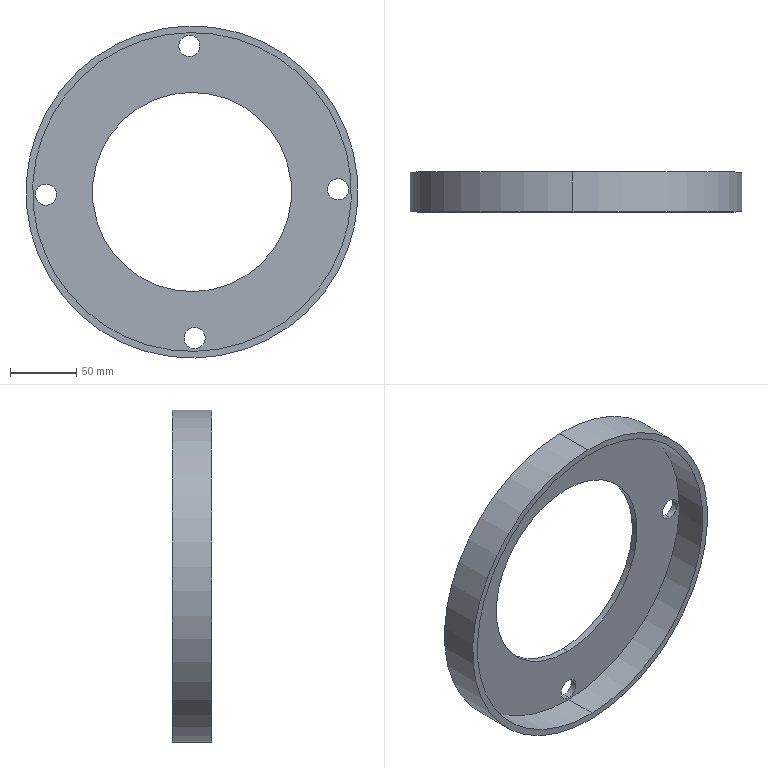Part | STEP file | 2026.6.15-Main Assembly图.sldasm-Part-1 | 1 solid | 17 faces | box 250 x 30 x 250 mm | volume 249270 mm3 | cylinder 14 | plane 3 | commonest cylinder face diameters 16 x8 150 x2 240 x2 250 x2
STEP:
#1=CARTESIAN_POINT('',(-752.482,776.976,3092.657));
#2=VERTEX_POINT('',#1);
#3=CARTESIAN_POINT('',(-752.191,776.976,3076.66));
#4=VERTEX_POINT('',#3);
#5=CARTESIAN_POINT('',(-752.337,776.976,3084.658));
#6=DIRECTION('',(0.,-1.,0.));
#7=DIRECTION('',(0.01819,0.,-0.9998));
#8=AXIS2_PLACEMENT_3D('',#5,#6,#7);
#9=CIRCLE('',#8,8.);
#10=EDGE_CURVE('',#2,#4,#9,.T.);
#11=ORIENTED_EDGE('',*,*,#10,.T.);
#12=CARTESIAN_POINT('',(-752.191,781.976,3076.66));
#13=VERTEX_POINT('',#12);
#14=CARTESIAN_POINT('',(-752.191,756.976,3076.66));
#15=DIRECTION('',(0.,-1.,0.));
#16=VECTOR('',#15,1000.);
#17=LINE('',#14,#16);
#18=EDGE_CURVE('',#13,#4,#17,.T.);
#19=ORIENTED_EDGE('',*,*,#18,.F.);
#20=CARTESIAN_POINT('',(-752.482,781.976,3092.657));
#21=VERTEX_POINT('',#20);
#22=CARTESIAN_POINT('',(-752.337,781.976,3084.658));
#23=DIRECTION('',(0.,1.,0.));
#24=DIRECTION('',(-0.01819,0.,0.9998));
#25=AXIS2_PLACEMENT_3D('',#22,#23,#24);
#26=CIRCLE('',#25,8.);
#27=EDGE_CURVE('',#13,#21,#26,.T.);
#28=ORIENTED_EDGE('',*,*,#27,.T.);
#29=CARTESIAN_POINT('',(-752.482,756.976,3092.657));
#30=DIRECTION('',(0.,-1.,0.));
#31=VECTOR('',#30,1000.);
#32=LINE('',#29,#31);
#33=EDGE_CURVE('',#21,#2,#32,.T.);
#34=ORIENTED_EDGE('',*,*,#33,.T.);
#35=EDGE_LOOP('',(#11,#19,#28,#34));
#36=FACE_OUTER_BOUND('',#35,.T.);
#37=CARTESIAN_POINT('',(-752.337,756.976,3084.658));
#38=DIRECTION('',(0.,1.,0.));
#39=DIRECTION('',(0.01819,0.,-0.9998));
#40=AXIS2_PLACEMENT_3D('',#37,#38,#39);
#41=CYLINDRICAL_SURFACE('',#40,8.);
#42=ADVANCED_FACE('',(#36),#41,.F.);
#43=CARTESIAN_POINT('',(-644.501,776.976,3204.639));
#44=VERTEX_POINT('',#43);
#45=CARTESIAN_POINT('',(-644.21,776.976,3188.642));
#46=VERTEX_POINT('',#45);
#47=CARTESIAN_POINT('',(-644.356,776.976,3196.641));
#48=DIRECTION('',(0.,-1.,0.));
#49=DIRECTION('',(0.01819,0.,-0.9998));
#50=AXIS2_PLACEMENT_3D('',#47,#48,#49);
#51=CIRCLE('',#50,8.);
#52=EDGE_CURVE('',#44,#46,#51,.T.);
#53=ORIENTED_EDGE('',*,*,#52,.T.);
#54=CARTESIAN_POINT('',(-644.21,781.976,3188.642));
#55=VERTEX_POINT('',#54);
#56=CARTESIAN_POINT('',(-644.21,756.976,3188.642));
#57=DIRECTION('',(0.,-1.,0.));
#58=VECTOR('',#57,1000.);
#59=LINE('',#56,#58);
#60=EDGE_CURVE('',#55,#46,#59,.T.);
#61=ORIENTED_EDGE('',*,*,#60,.F.);
#62=CARTESIAN_POINT('',(-644.501,781.976,3204.639));
#63=VERTEX_POINT('',#62);
#64=CARTESIAN_POINT('',(-644.356,781.976,3196.641));
#65=DIRECTION('',(0.,1.,0.));
#66=DIRECTION('',(-0.01819,0.,0.9998));
#67=AXIS2_PLACEMENT_3D('',#64,#65,#66);
#68=CIRCLE('',#67,8.);
#69=EDGE_CURVE('',#55,#63,#68,.T.);
#70=ORIENTED_EDGE('',*,*,#69,.T.);
#71=CARTESIAN_POINT('',(-644.501,756.976,3204.639));
#72=DIRECTION('',(0.,-1.,0.));
#73=VECTOR('',#72,1000.);
#74=LINE('',#71,#73);
#75=EDGE_CURVE('',#63,#44,#74,.T.);
#76=ORIENTED_EDGE('',*,*,#75,.T.);
#77=EDGE_LOOP('',(#53,#61,#70,#76));
#78=FACE_OUTER_BOUND('',#77,.T.);
#79=CARTESIAN_POINT('',(-644.356,756.976,3196.641));
#80=DIRECTION('',(0.,1.,0.));
#81=DIRECTION('',(0.01819,0.,-0.9998));
#82=AXIS2_PLACEMENT_3D('',#79,#80,#81);
#83=CYLINDRICAL_SURFACE('',#82,8.);
#84=ADVANCED_FACE('',(#78),#83,.F.);
#85=CARTESIAN_POINT('',(-864.465,776.976,3200.638));
#86=VERTEX_POINT('',#85);
#87=CARTESIAN_POINT('',(-864.174,776.976,3184.641));
#88=VERTEX_POINT('',#87);
#89=CARTESIAN_POINT('',(-864.319,776.976,3192.639));
#90=DIRECTION('',(0.,-1.,0.));
#91=DIRECTION('',(0.01819,0.,-0.9998));
#92=AXIS2_PLACEMENT_3D('',#89,#90,#91);
#93=CIRCLE('',#92,8.);
#94=EDGE_CURVE('',#86,#88,#93,.T.);
#95=ORIENTED_EDGE('',*,*,#94,.T.);
#96=CARTESIAN_POINT('',(-864.174,781.976,3184.641));
#97=VERTEX_POINT('',#96);
#98=CARTESIAN_POINT('',(-864.174,756.976,3184.641));
#99=DIRECTION('',(0.,-1.,0.));
#100=VECTOR('',#99,1000.);
#101=LINE('',#98,#100);
#102=EDGE_CURVE('',#97,#88,#101,.T.);
#103=ORIENTED_EDGE('',*,*,#102,.F.);
#104=CARTESIAN_POINT('',(-864.465,781.976,3200.638));
#105=VERTEX_POINT('',#104);
#106=CARTESIAN_POINT('',(-864.319,781.976,3192.639));
#107=DIRECTION('',(0.,1.,0.));
#108=DIRECTION('',(0.01819,0.,-0.9998));
#109=AXIS2_PLACEMENT_3D('',#106,#107,#108);
#110=CIRCLE('',#109,8.);
#111=EDGE_CURVE('',#97,#105,#110,.T.);
#112=ORIENTED_EDGE('',*,*,#111,.T.);
#113=CARTESIAN_POINT('',(-864.465,756.976,3200.638));
#114=DIRECTION('',(0.,-1.,0.));
#115=VECTOR('',#114,1000.);
#116=LINE('',#113,#115);
#117=EDGE_CURVE('',#105,#86,#116,.T.);
#118=ORIENTED_EDGE('',*,*,#117,.T.);
#119=EDGE_LOOP('',(#95,#103,#112,#118));
#120=FACE_OUTER_BOUND('',#119,.T.);
#121=CARTESIAN_POINT('',(-864.319,756.976,3192.639));
#122=DIRECTION('',(0.,1.,0.));
#123=DIRECTION('',(0.01819,0.,-0.9998));
#124=AXIS2_PLACEMENT_3D('',#121,#122,#123);
#125=CYLINDRICAL_SURFACE('',#124,8.);
#126=ADVANCED_FACE('',(#120),#125,.F.);
#127=CARTESIAN_POINT('',(-756.484,776.976,3312.621));
#128=VERTEX_POINT('',#127);
#129=CARTESIAN_POINT('',(-756.193,776.976,3296.623));
#130=VERTEX_POINT('',#129);
#131=CARTESIAN_POINT('',(-756.338,776.976,3304.622));
#132=DIRECTION('',(0.,-1.,0.));
#133=DIRECTION('',(0.01819,0.,-0.9998));
#134=AXIS2_PLACEMENT_3D('',#131,#132,#133);
#135=CIRCLE('',#134,8.);
#136=EDGE_CURVE('',#128,#130,#135,.T.);
#137=ORIENTED_EDGE('',*,*,#136,.T.);
#138=CARTESIAN_POINT('',(-756.193,781.976,3296.623));
#139=VERTEX_POINT('',#138);
#140=CARTESIAN_POINT('',(-756.193,756.976,3296.623));
#141=DIRECTION('',(0.,-1.,0.));
#142=VECTOR('',#141,1000.);
#143=LINE('',#140,#142);
#144=EDGE_CURVE('',#139,#130,#143,.T.);
#145=ORIENTED_EDGE('',*,*,#144,.F.);
#146=CARTESIAN_POINT('',(-756.484,781.976,3312.621));
#147=VERTEX_POINT('',#146);
#148=CARTESIAN_POINT('',(-756.338,781.976,3304.622));
#149=DIRECTION('',(0.,1.,0.));
#150=DIRECTION('',(0.01819,0.,-0.9998));
#151=AXIS2_PLACEMENT_3D('',#148,#149,#150);
#152=CIRCLE('',#151,8.);
#153=EDGE_CURVE('',#139,#147,#152,.T.);
#154=ORIENTED_EDGE('',*,*,#153,.T.);
#155=CARTESIAN_POINT('',(-756.484,756.976,3312.621));
#156=DIRECTION('',(0.,-1.,0.));
#157=VECTOR('',#156,1000.);
#158=LINE('',#155,#157);
#159=EDGE_CURVE('',#147,#128,#158,.T.);
#160=ORIENTED_EDGE('',*,*,#159,.T.);
#161=EDGE_LOOP('',(#137,#145,#154,#160));
#162=FACE_OUTER_BOUND('',#161,.T.);
#163=CARTESIAN_POINT('',(-756.338,756.976,3304.622));
#164=DIRECTION('',(0.,1.,0.));
#165=DIRECTION('',(0.01819,0.,-0.9998));
#166=AXIS2_PLACEMENT_3D('',#163,#164,#165);
#167=CYLINDRICAL_SURFACE('',#166,8.);
#168=ADVANCED_FACE('',(#162),#167,.F.);
#169=CARTESIAN_POINT('',(-756.52,776.976,3314.62));
#170=VERTEX_POINT('',#169);
#171=CARTESIAN_POINT('',(-752.155,776.976,3074.66));
#172=VERTEX_POINT('',#171);
#173=CARTESIAN_POINT('',(-754.337,776.976,3194.64));
#174=DIRECTION('',(0.,-1.,0.));
#175=DIRECTION('',(0.01819,0.,-0.9998));
#176=AXIS2_PLACEMENT_3D('',#173,#174,#175);
#177=CIRCLE('',#176,120.);
#178=EDGE_CURVE('',#170,#172,#177,.T.);
#179=ORIENTED_EDGE('',*,*,#178,.F.);
#180=CARTESIAN_POINT('',(-756.52,751.976,3314.62));
#181=VERTEX_POINT('',#180);
#182=CARTESIAN_POINT('',(-756.52,776.976,3314.62));
#183=DIRECTION('',(0.,-1.,0.));
#184=VECTOR('',#183,1000.);
#185=LINE('',#182,#184);
#186=EDGE_CURVE('',#170,#181,#185,.T.);
#187=ORIENTED_EDGE('',*,*,#186,.T.);
#188=CARTESIAN_POINT('',(-752.155,751.976,3074.66));
#189=VERTEX_POINT('',#188);
#190=CARTESIAN_POINT('',(-754.337,751.976,3194.64));
#191=DIRECTION('',(0.,-1.,0.));
#192=DIRECTION('',(0.01819,0.,-0.9998));
#193=AXIS2_PLACEMENT_3D('',#190,#191,#192);
#194=CIRCLE('',#193,120.);
#195=EDGE_CURVE('',#181,#189,#194,.T.);
#196=ORIENTED_EDGE('',*,*,#195,.T.);
#197=CARTESIAN_POINT('',(-752.155,776.976,3074.66));
#198=DIRECTION('',(0.,-1.,0.));
#199=VECTOR('',#198,1000.);
#200=LINE('',#197,#199);
#201=EDGE_CURVE('',#172,#189,#200,.T.);
#202=ORIENTED_EDGE('',*,*,#201,.F.);
#203=EDGE_LOOP('',(#179,#187,#196,#202));
#204=FACE_OUTER_BOUND('',#203,.T.);
#205=CARTESIAN_POINT('',(-754.337,776.976,3194.64));
#206=DIRECTION('',(0.,-1.,0.));
#207=DIRECTION('',(-0.01819,0.,0.9998));
#208=AXIS2_PLACEMENT_3D('',#205,#206,#207);
#209=CYLINDRICAL_SURFACE('',#208,120.);
#210=ADVANCED_FACE('',(#204),#209,.F.);
#211=CARTESIAN_POINT('',(-752.064,751.976,3069.661));
#212=VERTEX_POINT('',#211);
#213=CARTESIAN_POINT('',(-756.611,751.976,3319.619));
#214=VERTEX_POINT('',#213);
#215=CARTESIAN_POINT('',(-754.337,751.976,3194.64));
#216=DIRECTION('',(0.,-1.,0.));
#217=DIRECTION('',(0.01819,0.,-0.9998));
#218=AXIS2_PLACEMENT_3D('',#215,#216,#217);
#219=CIRCLE('',#218,125.);
#220=EDGE_CURVE('',#212,#214,#219,.T.);
#221=ORIENTED_EDGE('',*,*,#220,.F.);
#222=CARTESIAN_POINT('',(-752.064,781.976,3069.661));
#223=VERTEX_POINT('',#222);
#224=CARTESIAN_POINT('',(-752.064,751.976,3069.661));
#225=DIRECTION('',(0.,-1.,0.));
#226=VECTOR('',#225,1000.);
#227=LINE('',#224,#226);
#228=EDGE_CURVE('',#223,#212,#227,.T.);
#229=ORIENTED_EDGE('',*,*,#228,.F.);
#230=CARTESIAN_POINT('',(-756.611,781.976,3319.619));
#231=VERTEX_POINT('',#230);
#232=CARTESIAN_POINT('',(-754.337,781.976,3194.64));
#233=DIRECTION('',(0.,-1.,0.));
#234=DIRECTION('',(0.01819,0.,-0.9998));
#235=AXIS2_PLACEMENT_3D('',#232,#233,#234);
#236=CIRCLE('',#235,125.);
#237=EDGE_CURVE('',#223,#231,#236,.T.);
#238=ORIENTED_EDGE('',*,*,#237,.T.);
#239=CARTESIAN_POINT('',(-756.611,751.976,3319.619));
#240=DIRECTION('',(0.,-1.,0.));
#241=VECTOR('',#240,1000.);
#242=LINE('',#239,#241);
#243=EDGE_CURVE('',#231,#214,#242,.T.);
#244=ORIENTED_EDGE('',*,*,#243,.T.);
#245=EDGE_LOOP('',(#221,#229,#238,#244));
#246=FACE_OUTER_BOUND('',#245,.T.);
#247=CARTESIAN_POINT('',(-754.337,751.976,3194.64));
#248=DIRECTION('',(0.,1.,0.));
#249=DIRECTION('',(0.01819,0.,-0.9998));
#250=AXIS2_PLACEMENT_3D('',#247,#248,#249);
#251=CYLINDRICAL_SURFACE('',#250,125.);
#252=ADVANCED_FACE('',(#246),#251,.T.);
#253=CARTESIAN_POINT('',(-755.702,776.976,3269.628));
#254=VERTEX_POINT('',#253);
#255=CARTESIAN_POINT('',(-752.973,776.976,3119.652));
#256=VERTEX_POINT('',#255);
#257=CARTESIAN_POINT('',(-754.337,776.976,3194.64));
#258=DIRECTION('',(0.,-1.,0.));
#259=DIRECTION('',(0.01819,0.,-0.9998));
#260=AXIS2_PLACEMENT_3D('',#257,#258,#259);
#261=CIRCLE('',#260,75.);
#262=EDGE_CURVE('',#254,#256,#261,.T.);
#263=ORIENTED_EDGE('',*,*,#262,.T.);
#264=CARTESIAN_POINT('',(-752.973,781.976,3119.652));
#265=VERTEX_POINT('',#264);
#266=CARTESIAN_POINT('',(-752.973,751.976,3119.652));
#267=DIRECTION('',(0.,-1.,0.));
#268=VECTOR('',#267,1000.);
#269=LINE('',#266,#268);
#270=EDGE_CURVE('',#265,#256,#269,.T.);
#271=ORIENTED_EDGE('',*,*,#270,.F.);
#272=CARTESIAN_POINT('',(-755.702,781.976,3269.628));
#273=VERTEX_POINT('',#272);
#274=CARTESIAN_POINT('',(-754.337,781.976,3194.64));
#275=DIRECTION('',(0.,-1.,0.));
#276=DIRECTION('',(0.01819,0.,-0.9998));
#277=AXIS2_PLACEMENT_3D('',#274,#275,#276);
#278=CIRCLE('',#277,75.);
#279=EDGE_CURVE('',#273,#265,#278,.T.);
#280=ORIENTED_EDGE('',*,*,#279,.F.);
#281=CARTESIAN_POINT('',(-755.702,751.976,3269.628));
#282=DIRECTION('',(0.,-1.,0.));
#283=VECTOR('',#282,1000.);
#284=LINE('',#281,#283);
#285=EDGE_CURVE('',#273,#254,#284,.T.);
#286=ORIENTED_EDGE('',*,*,#285,.T.);
#287=EDGE_LOOP('',(#263,#271,#280,#286));
#288=FACE_OUTER_BOUND('',#287,.T.);
#289=CARTESIAN_POINT('',(-754.337,751.976,3194.64));
#290=DIRECTION('',(0.,1.,0.));
#291=DIRECTION('',(0.01819,0.,-0.9998));
#292=AXIS2_PLACEMENT_3D('',#289,#290,#291);
#293=CYLINDRICAL_SURFACE('',#292,75.);
#294=ADVANCED_FACE('',(#288),#293,.F.);
#295=ORIENTED_EDGE('',*,*,#270,.T.);
#296=CARTESIAN_POINT('',(-754.337,776.976,3194.64));
#297=DIRECTION('',(0.,-1.,0.));
#298=DIRECTION('',(0.01819,0.,-0.9998));
#299=AXIS2_PLACEMENT_3D('',#296,#297,#298);
#300=CIRCLE('',#299,75.);
#301=EDGE_CURVE('',#256,#254,#300,.T.);
#302=ORIENTED_EDGE('',*,*,#301,.T.);
#303=ORIENTED_EDGE('',*,*,#285,.F.);
#304=CARTESIAN_POINT('',(-754.337,781.976,3194.64));
#305=DIRECTION('',(0.,-1.,0.));
#306=DIRECTION('',(0.01819,0.,-0.9998));
#307=AXIS2_PLACEMENT_3D('',#304,#305,#306);
#308=CIRCLE('',#307,75.);
#309=EDGE_CURVE('',#265,#273,#308,.T.);
#310=ORIENTED_EDGE('',*,*,#309,.F.);
#311=EDGE_LOOP('',(#295,#302,#303,#310));
#312=FACE_OUTER_BOUND('',#311,.T.);
#313=CARTESIAN_POINT('',(-754.337,751.976,3194.64));
#314=DIRECTION('',(0.,1.,0.));
#315=DIRECTION('',(0.01819,0.,-0.9998));
#316=AXIS2_PLACEMENT_3D('',#313,#314,#315);
#317=CYLINDRICAL_SURFACE('',#316,75.);
#318=ADVANCED_FACE('',(#312),#317,.F.);
#319=CARTESIAN_POINT('',(-754.337,751.976,3194.64));
#320=DIRECTION('',(0.,-1.,0.));
#321=DIRECTION('',(0.01819,0.,-0.9998));
#322=AXIS2_PLACEMENT_3D('',#319,#320,#321);
#323=CIRCLE('',#322,125.);
#324=EDGE_CURVE('',#214,#212,#323,.T.);
#325=ORIENTED_EDGE('',*,*,#324,.T.);
#326=ORIENTED_EDGE('',*,*,#220,.T.);
#327=EDGE_LOOP('',(#325,#326));
#328=FACE_OUTER_BOUND('',#327,.T.);
#329=CARTESIAN_POINT('',(-754.337,751.976,3194.64));
#330=DIRECTION('',(0.,-1.,0.));
#331=DIRECTION('',(0.01819,0.,-0.9998));
#332=AXIS2_PLACEMENT_3D('',#329,#330,#331);
#333=CIRCLE('',#332,120.);
#334=EDGE_CURVE('',#189,#181,#333,.T.);
#335=ORIENTED_EDGE('',*,*,#334,.F.);
#336=ORIENTED_EDGE('',*,*,#195,.F.);
#337=EDGE_LOOP('',(#335,#336));
#338=FACE_BOUND('',#337,.T.);
#339=CARTESIAN_POINT('',(-754.337,751.976,3194.64));
#340=DIRECTION('',(0.,-1.,0.));
#341=DIRECTION('',(-0.9998,0.,-0.01819));
#342=AXIS2_PLACEMENT_3D('',#339,#340,#341);
#343=PLANE('',#342);
#344=ADVANCED_FACE('',(#328,#338),#343,.T.);
#345=CARTESIAN_POINT('',(-754.337,781.976,3194.64));
#346=DIRECTION('',(0.,-1.,0.));
#347=DIRECTION('',(0.01819,0.,-0.9998));
#348=AXIS2_PLACEMENT_3D('',#345,#346,#347);
#349=CIRCLE('',#348,125.);
#350=EDGE_CURVE('',#231,#223,#349,.T.);
#351=ORIENTED_EDGE('',*,*,#350,.F.);
#352=ORIENTED_EDGE('',*,*,#237,.F.);
#353=EDGE_LOOP('',(#351,#352));
#354=FACE_OUTER_BOUND('',#353,.T.);
#355=CARTESIAN_POINT('',(-752.337,781.976,3084.658));
#356=DIRECTION('',(0.,1.,0.));
#357=DIRECTION('',(-0.01819,0.,0.9998));
#358=AXIS2_PLACEMENT_3D('',#355,#356,#357);
#359=CIRCLE('',#358,8.);
#360=EDGE_CURVE('',#21,#13,#359,.T.);
#361=ORIENTED_EDGE('',*,*,#360,.F.);
#362=ORIENTED_EDGE('',*,*,#27,.F.);
#363=EDGE_LOOP('',(#361,#362));
#364=FACE_BOUND('',#363,.T.);
#365=CARTESIAN_POINT('',(-644.356,781.976,3196.641));
#366=DIRECTION('',(0.,1.,0.));
#367=DIRECTION('',(-0.01819,0.,0.9998));
#368=AXIS2_PLACEMENT_3D('',#365,#366,#367);
#369=CIRCLE('',#368,8.);
#370=EDGE_CURVE('',#63,#55,#369,.T.);
#371=ORIENTED_EDGE('',*,*,#370,.F.);
#372=ORIENTED_EDGE('',*,*,#69,.F.);
#373=EDGE_LOOP('',(#371,#372));
#374=FACE_BOUND('',#373,.T.);
#375=CARTESIAN_POINT('',(-864.319,781.976,3192.639));
#376=DIRECTION('',(0.,1.,0.));
#377=DIRECTION('',(0.01819,0.,-0.9998));
#378=AXIS2_PLACEMENT_3D('',#375,#376,#377);
#379=CIRCLE('',#378,8.);
#380=EDGE_CURVE('',#105,#97,#379,.T.);
#381=ORIENTED_EDGE('',*,*,#380,.F.);
#382=ORIENTED_EDGE('',*,*,#111,.F.);
#383=EDGE_LOOP('',(#381,#382));
#384=FACE_BOUND('',#383,.T.);
#385=CARTESIAN_POINT('',(-756.338,781.976,3304.622));
#386=DIRECTION('',(0.,1.,0.));
#387=DIRECTION('',(0.01819,0.,-0.9998));
#388=AXIS2_PLACEMENT_3D('',#385,#386,#387);
#389=CIRCLE('',#388,8.);
#390=EDGE_CURVE('',#147,#139,#389,.T.);
#391=ORIENTED_EDGE('',*,*,#390,.F.);
#392=ORIENTED_EDGE('',*,*,#153,.F.);
#393=EDGE_LOOP('',(#391,#392));
#394=FACE_BOUND('',#393,.T.);
#395=ORIENTED_EDGE('',*,*,#279,.T.);
#396=ORIENTED_EDGE('',*,*,#309,.T.);
#397=EDGE_LOOP('',(#395,#396));
#398=FACE_BOUND('',#397,.T.);
#399=CARTESIAN_POINT('',(-754.337,781.976,3194.64));
#400=DIRECTION('',(0.,-1.,0.));
#401=DIRECTION('',(-0.9998,0.,-0.01819));
#402=AXIS2_PLACEMENT_3D('',#399,#400,#401);
#403=PLANE('',#402);
#404=ADVANCED_FACE('',(#354,#364,#374,#384,#394,#398),#403,.F.);
#405=ORIENTED_EDGE('',*,*,#228,.T.);
#406=ORIENTED_EDGE('',*,*,#324,.F.);
#407=ORIENTED_EDGE('',*,*,#243,.F.);
#408=ORIENTED_EDGE('',*,*,#350,.T.);
#409=EDGE_LOOP('',(#405,#406,#407,#408));
#410=FACE_OUTER_BOUND('',#409,.T.);
#411=CARTESIAN_POINT('',(-754.337,751.976,3194.64));
#412=DIRECTION('',(0.,1.,0.));
#413=DIRECTION('',(0.01819,0.,-0.9998));
#414=AXIS2_PLACEMENT_3D('',#411,#412,#413);
#415=CYLINDRICAL_SURFACE('',#414,125.);
#416=ADVANCED_FACE('',(#410),#415,.T.);
#417=ORIENTED_EDGE('',*,*,#186,.F.);
#418=CARTESIAN_POINT('',(-754.337,776.976,3194.64));
#419=DIRECTION('',(0.,-1.,0.));
#420=DIRECTION('',(0.01819,0.,-0.9998));
#421=AXIS2_PLACEMENT_3D('',#418,#419,#420);
#422=CIRCLE('',#421,120.);
#423=EDGE_CURVE('',#172,#170,#422,.T.);
#424=ORIENTED_EDGE('',*,*,#423,.F.);
#425=ORIENTED_EDGE('',*,*,#201,.T.);
#426=ORIENTED_EDGE('',*,*,#334,.T.);
#427=EDGE_LOOP('',(#417,#424,#425,#426));
#428=FACE_OUTER_BOUND('',#427,.T.);
#429=CARTESIAN_POINT('',(-754.337,776.976,3194.64));
#430=DIRECTION('',(0.,-1.,0.));
#431=DIRECTION('',(-0.01819,0.,0.9998));
#432=AXIS2_PLACEMENT_3D('',#429,#430,#431);
#433=CYLINDRICAL_SURFACE('',#432,120.);
#434=ADVANCED_FACE('',(#428),#433,.F.);
#435=ORIENTED_EDGE('',*,*,#423,.T.);
#436=ORIENTED_EDGE('',*,*,#178,.T.);
#437=EDGE_LOOP('',(#435,#436));
#438=FACE_OUTER_BOUND('',#437,.T.);
#439=ORIENTED_EDGE('',*,*,#10,.F.);
#440=CARTESIAN_POINT('',(-752.337,776.976,3084.658));
#441=DIRECTION('',(0.,-1.,0.));
#442=DIRECTION('',(0.01819,0.,-0.9998));
#443=AXIS2_PLACEMENT_3D('',#440,#441,#442);
#444=CIRCLE('',#443,8.);
#445=EDGE_CURVE('',#4,#2,#444,.T.);
#446=ORIENTED_EDGE('',*,*,#445,.F.);
#447=EDGE_LOOP('',(#439,#446));
#448=FACE_BOUND('',#447,.T.);
#449=ORIENTED_EDGE('',*,*,#52,.F.);
#450=CARTESIAN_POINT('',(-644.356,776.976,3196.641));
#451=DIRECTION('',(0.,-1.,0.));
#452=DIRECTION('',(0.01819,0.,-0.9998));
#453=AXIS2_PLACEMENT_3D('',#450,#451,#452);
#454=CIRCLE('',#453,8.);
#455=EDGE_CURVE('',#46,#44,#454,.T.);
#456=ORIENTED_EDGE('',*,*,#455,.F.);
#457=EDGE_LOOP('',(#449,#456));
#458=FACE_BOUND('',#457,.T.);
#459=ORIENTED_EDGE('',*,*,#94,.F.);
#460=CARTESIAN_POINT('',(-864.319,776.976,3192.639));
#461=DIRECTION('',(0.,-1.,0.));
#462=DIRECTION('',(0.01819,0.,-0.9998));
#463=AXIS2_PLACEMENT_3D('',#460,#461,#462);
#464=CIRCLE('',#463,8.);
#465=EDGE_CURVE('',#88,#86,#464,.T.);
#466=ORIENTED_EDGE('',*,*,#465,.F.);
#467=EDGE_LOOP('',(#459,#466));
#468=FACE_BOUND('',#467,.T.);
#469=ORIENTED_EDGE('',*,*,#136,.F.);
#470=CARTESIAN_POINT('',(-756.338,776.976,3304.622));
#471=DIRECTION('',(0.,-1.,0.));
#472=DIRECTION('',(0.01819,0.,-0.9998));
#473=AXIS2_PLACEMENT_3D('',#470,#471,#472);
#474=CIRCLE('',#473,8.);
#475=EDGE_CURVE('',#130,#128,#474,.T.);
#476=ORIENTED_EDGE('',*,*,#475,.F.);
#477=EDGE_LOOP('',(#469,#476));
#478=FACE_BOUND('',#477,.T.);
#479=ORIENTED_EDGE('',*,*,#262,.F.);
#480=ORIENTED_EDGE('',*,*,#301,.F.);
#481=EDGE_LOOP('',(#479,#480));
#482=FACE_BOUND('',#481,.T.);
#483=CARTESIAN_POINT('',(-754.337,776.976,3194.64));
#484=DIRECTION('',(0.,-1.,0.));
#485=DIRECTION('',(-0.9998,0.,-0.01819));
#486=AXIS2_PLACEMENT_3D('',#483,#484,#485);
#487=PLANE('',#486);
#488=ADVANCED_FACE('',(#438,#448,#458,#468,#478,#482),#487,.T.);
#489=ORIENTED_EDGE('',*,*,#144,.T.);
#490=ORIENTED_EDGE('',*,*,#475,.T.);
#491=ORIENTED_EDGE('',*,*,#159,.F.);
#492=ORIENTED_EDGE('',*,*,#390,.T.);
#493=EDGE_LOOP('',(#489,#490,#491,#492));
#494=FACE_OUTER_BOUND('',#493,.T.);
#495=CARTESIAN_POINT('',(-756.338,756.976,3304.622));
#496=DIRECTION('',(0.,1.,0.));
#497=DIRECTION('',(0.01819,0.,-0.9998));
#498=AXIS2_PLACEMENT_3D('',#495,#496,#497);
#499=CYLINDRICAL_SURFACE('',#498,8.);
#500=ADVANCED_FACE('',(#494),#499,.F.);
#501=ORIENTED_EDGE('',*,*,#102,.T.);
#502=ORIENTED_EDGE('',*,*,#465,.T.);
#503=ORIENTED_EDGE('',*,*,#117,.F.);
#504=ORIENTED_EDGE('',*,*,#380,.T.);
#505=EDGE_LOOP('',(#501,#502,#503,#504));
#506=FACE_OUTER_BOUND('',#505,.T.);
#507=CARTESIAN_POINT('',(-864.319,756.976,3192.639));
#508=DIRECTION('',(0.,1.,0.));
#509=DIRECTION('',(0.01819,0.,-0.9998));
#510=AXIS2_PLACEMENT_3D('',#507,#508,#509);
#511=CYLINDRICAL_SURFACE('',#510,8.);
#512=ADVANCED_FACE('',(#506),#511,.F.);
#513=ORIENTED_EDGE('',*,*,#60,.T.);
#514=ORIENTED_EDGE('',*,*,#455,.T.);
#515=ORIENTED_EDGE('',*,*,#75,.F.);
#516=ORIENTED_EDGE('',*,*,#370,.T.);
#517=EDGE_LOOP('',(#513,#514,#515,#516));
#518=FACE_OUTER_BOUND('',#517,.T.);
#519=CARTESIAN_POINT('',(-644.356,756.976,3196.641));
#520=DIRECTION('',(0.,1.,0.));
#521=DIRECTION('',(0.01819,0.,-0.9998));
#522=AXIS2_PLACEMENT_3D('',#519,#520,#521);
#523=CYLINDRICAL_SURFACE('',#522,8.);
#524=ADVANCED_FACE('',(#518),#523,.F.);
#525=ORIENTED_EDGE('',*,*,#18,.T.);
#526=ORIENTED_EDGE('',*,*,#445,.T.);
#527=ORIENTED_EDGE('',*,*,#33,.F.);
#528=ORIENTED_EDGE('',*,*,#360,.T.);
#529=EDGE_LOOP('',(#525,#526,#527,#528));
#530=FACE_OUTER_BOUND('',#529,.T.);
#531=CARTESIAN_POINT('',(-752.337,756.976,3084.658));
#532=DIRECTION('',(0.,1.,0.));
#533=DIRECTION('',(0.01819,0.,-0.9998));
#534=AXIS2_PLACEMENT_3D('',#531,#532,#533);
#535=CYLINDRICAL_SURFACE('',#534,8.);
#536=ADVANCED_FACE('',(#530),#535,.F.);
#537=CLOSED_SHELL('',(#42,#84,#126,#168,#210,#252,#294,#318,#344,#404,#416,#434,#488,#500,#512,#524,#536));
#538=MANIFOLD_SOLID_BREP('',#537);
#539=CARTESIAN_POINT('',(0.,0.,0.));
#540=DIRECTION('',(0.,0.,1.));
#541=DIRECTION('',(1.,0.,0.));
#542=AXIS2_PLACEMENT_3D('',#539,#540,#541);
#543=(LENGTH_UNIT()NAMED_UNIT(*)SI_UNIT(.MILLI.,.METRE.));
#544=UNCERTAINTY_MEASURE_WITH_UNIT(LENGTH_MEASURE(0.00001),#543,'','');
#545=(NAMED_UNIT(*)PLANE_ANGLE_UNIT()SI_UNIT($,.RADIAN.));
#546=(NAMED_UNIT(*)SI_UNIT($,.STERADIAN.)SOLID_ANGLE_UNIT());
#547=(GEOMETRIC_REPRESENTATION_CONTEXT(3)GLOBAL_UNCERTAINTY_ASSIGNED_CONTEXT((#544))GLOBAL_UNIT_ASSIGNED_CONTEXT((#543,#545,#546))REPRESENTATION_CONTEXT('',''));
#548=ADVANCED_BREP_SHAPE_REPRESENTATION('',(#538,#542),#547);